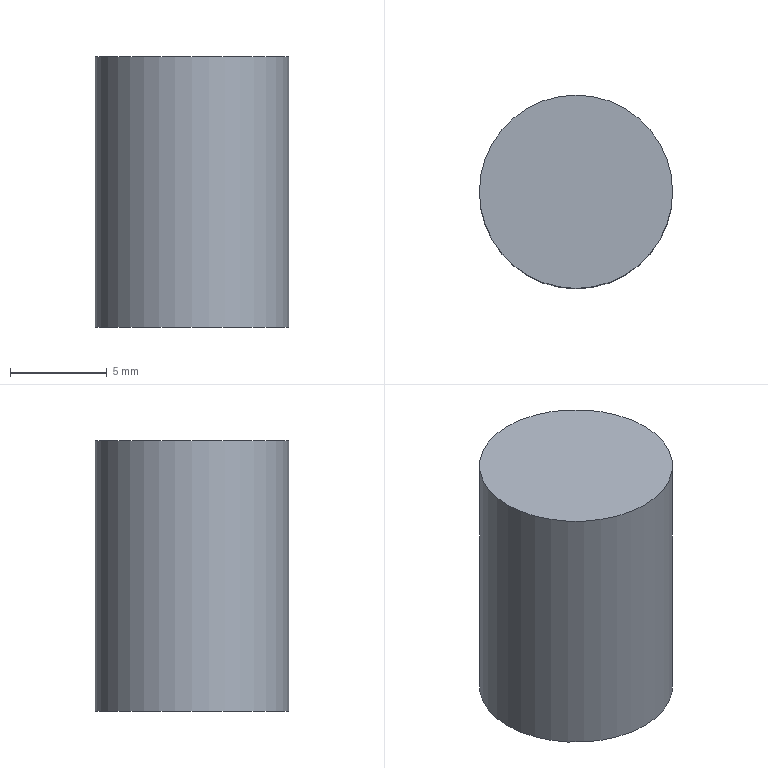Part | NX | features solid 2 | 1 solid | 3 faces | box 10 x 10 x 14 mm | volume 1100 mm3 | plane 2 | cylinder 1 | commonest cylinder face diameters 10 x1
STEP:
#1=CARTESIAN_POINT('',(50.,-415.,-188.));
#2=VERTEX_POINT('',#1);
#3=CARTESIAN_POINT('',(55.,-415.,-188.));
#4=DIRECTION('',(0.,0.,-1.));
#5=DIRECTION('',(-1.,0.,0.));
#6=AXIS2_PLACEMENT_3D('',#3,#4,#5);
#7=CIRCLE('',#6,5.);
#8=EDGE_CURVE('',#2,#2,#7,.T.);
#9=ORIENTED_EDGE('',*,*,#8,.F.);
#10=EDGE_LOOP('',(#9));
#11=FACE_BOUND('',#10,.T.);
#12=CARTESIAN_POINT('',(50.,-415.,-174.));
#13=VERTEX_POINT('',#12);
#14=CARTESIAN_POINT('',(55.,-415.,-174.));
#15=DIRECTION('',(0.,0.,-1.));
#16=DIRECTION('',(-1.,0.,0.));
#17=AXIS2_PLACEMENT_3D('',#14,#15,#16);
#18=CIRCLE('',#17,5.);
#19=EDGE_CURVE('',#13,#13,#18,.T.);
#20=ORIENTED_EDGE('',*,*,#19,.T.);
#21=EDGE_LOOP('',(#20));
#22=FACE_BOUND('',#21,.T.);
#23=CARTESIAN_POINT('',(55.,-415.,-188.));
#24=DIRECTION('',(0.,0.,1.));
#25=DIRECTION('',(-1.,0.,0.));
#26=AXIS2_PLACEMENT_3D('',#23,#24,#25);
#27=CYLINDRICAL_SURFACE('',#26,5.);
#28=ADVANCED_FACE('',(#11,#22),#27,.T.);
#29=ORIENTED_EDGE('',*,*,#8,.T.);
#30=EDGE_LOOP('',(#29));
#31=FACE_BOUND('',#30,.T.);
#32=CARTESIAN_POINT('',(55.,-415.,-188.));
#33=DIRECTION('',(0.,0.,1.));
#34=DIRECTION('',(-1.,0.,0.));
#35=AXIS2_PLACEMENT_3D('',#32,#33,#34);
#36=PLANE('',#35);
#37=ADVANCED_FACE('',(#31),#36,.F.);
#38=ORIENTED_EDGE('',*,*,#19,.F.);
#39=EDGE_LOOP('',(#38));
#40=FACE_BOUND('',#39,.T.);
#41=CARTESIAN_POINT('',(55.,-415.,-174.));
#42=DIRECTION('',(0.,0.,1.));
#43=DIRECTION('',(-1.,0.,0.));
#44=AXIS2_PLACEMENT_3D('',#41,#42,#43);
#45=PLANE('',#44);
#46=ADVANCED_FACE('',(#40),#45,.T.);
#47=CLOSED_SHELL('',(#28,#37,#46));
#48=MANIFOLD_SOLID_BREP('',#47);
#49=(LENGTH_UNIT()NAMED_UNIT(*)SI_UNIT(.MILLI.,.METRE.));
#50=UNCERTAINTY_MEASURE_WITH_UNIT(LENGTH_MEASURE(0.00001),#49,'','');
#51=(NAMED_UNIT(*)PLANE_ANGLE_UNIT()SI_UNIT($,.RADIAN.));
#52=(NAMED_UNIT(*)SI_UNIT($,.STERADIAN.)SOLID_ANGLE_UNIT());
#53=(GEOMETRIC_REPRESENTATION_CONTEXT(3)GLOBAL_UNCERTAINTY_ASSIGNED_CONTEXT((#50))GLOBAL_UNIT_ASSIGNED_CONTEXT((#49,#51,#52))REPRESENTATION_CONTEXT('',''));
#54=ADVANCED_BREP_SHAPE_REPRESENTATION('',(#48),#53);